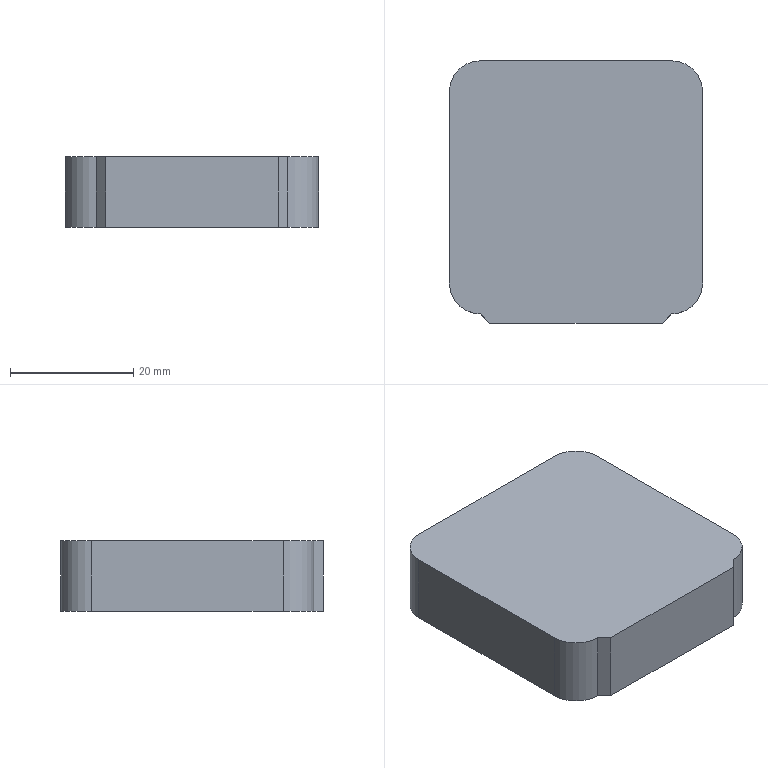Part | SolidWorks | features BaseBody 1 | 1 solid | 12 faces | box 41 x 42.5 x 11.5 mm | volume 19594 mm3 | plane 8 | cylinder 4 | commonest cylinder face diameters 10 x4
STEP:
#1=CARTESIAN_POINT('',(-10.199,-21.152,0.));
#2=VERTEX_POINT('',#1);
#3=CARTESIAN_POINT('',(17.801,-21.152,0.));
#4=VERTEX_POINT('',#3);
#5=CARTESIAN_POINT('',(3.801,-21.152,0.));
#6=DIRECTION('',(1.,0.,0.));
#7=VECTOR('',#6,1000.);
#8=LINE('',#5,#7);
#9=EDGE_CURVE('',#2,#4,#8,.T.);
#10=ORIENTED_EDGE('',*,*,#9,.F.);
#11=CARTESIAN_POINT('',(-11.699,-19.652,0.));
#12=VERTEX_POINT('',#11);
#13=CARTESIAN_POINT('',(-11.699,-19.652,0.));
#14=DIRECTION('',(0.7071,-0.7071,0.));
#15=VECTOR('',#14,1000.);
#16=LINE('',#13,#15);
#17=EDGE_CURVE('',#12,#2,#16,.T.);
#18=ORIENTED_EDGE('',*,*,#17,.F.);
#19=CARTESIAN_POINT('',(-16.699,-14.652,0.));
#20=VERTEX_POINT('',#19);
#21=CARTESIAN_POINT('',(-11.699,-14.652,0.));
#22=DIRECTION('',(0.,0.,1.));
#23=DIRECTION('',(1.,0.,0.));
#24=AXIS2_PLACEMENT_3D('',#21,#22,#23);
#25=CIRCLE('',#24,5.);
#26=EDGE_CURVE('',#20,#12,#25,.T.);
#27=ORIENTED_EDGE('',*,*,#26,.F.);
#28=CARTESIAN_POINT('',(-16.699,16.348,0.));
#29=VERTEX_POINT('',#28);
#30=CARTESIAN_POINT('',(-16.699,0.8485,0.));
#31=DIRECTION('',(0.,-1.,0.));
#32=VECTOR('',#31,1000.);
#33=LINE('',#30,#32);
#34=EDGE_CURVE('',#29,#20,#33,.T.);
#35=ORIENTED_EDGE('',*,*,#34,.F.);
#36=CARTESIAN_POINT('',(-11.699,21.348,0.));
#37=VERTEX_POINT('',#36);
#38=CARTESIAN_POINT('',(-11.699,16.348,0.));
#39=DIRECTION('',(0.,0.,1.));
#40=DIRECTION('',(1.,0.,0.));
#41=AXIS2_PLACEMENT_3D('',#38,#39,#40);
#42=CIRCLE('',#41,5.);
#43=EDGE_CURVE('',#37,#29,#42,.T.);
#44=ORIENTED_EDGE('',*,*,#43,.F.);
#45=CARTESIAN_POINT('',(19.301,21.348,0.));
#46=VERTEX_POINT('',#45);
#47=CARTESIAN_POINT('',(3.801,21.348,0.));
#48=DIRECTION('',(-1.,0.,0.));
#49=VECTOR('',#48,1000.);
#50=LINE('',#47,#49);
#51=EDGE_CURVE('',#46,#37,#50,.T.);
#52=ORIENTED_EDGE('',*,*,#51,.F.);
#53=CARTESIAN_POINT('',(24.301,16.348,0.));
#54=VERTEX_POINT('',#53);
#55=CARTESIAN_POINT('',(19.301,16.348,0.));
#56=DIRECTION('',(0.,0.,1.));
#57=DIRECTION('',(1.,0.,0.));
#58=AXIS2_PLACEMENT_3D('',#55,#56,#57);
#59=CIRCLE('',#58,5.);
#60=EDGE_CURVE('',#54,#46,#59,.T.);
#61=ORIENTED_EDGE('',*,*,#60,.F.);
#62=CARTESIAN_POINT('',(24.301,-14.652,0.));
#63=VERTEX_POINT('',#62);
#64=CARTESIAN_POINT('',(24.301,0.8485,0.));
#65=DIRECTION('',(0.,1.,0.));
#66=VECTOR('',#65,1000.);
#67=LINE('',#64,#66);
#68=EDGE_CURVE('',#63,#54,#67,.T.);
#69=ORIENTED_EDGE('',*,*,#68,.F.);
#70=CARTESIAN_POINT('',(19.301,-19.652,0.));
#71=VERTEX_POINT('',#70);
#72=CARTESIAN_POINT('',(19.301,-14.652,0.));
#73=DIRECTION('',(0.,0.,1.));
#74=DIRECTION('',(1.,0.,0.));
#75=AXIS2_PLACEMENT_3D('',#72,#73,#74);
#76=CIRCLE('',#75,5.);
#77=EDGE_CURVE('',#71,#63,#76,.T.);
#78=ORIENTED_EDGE('',*,*,#77,.F.);
#79=CARTESIAN_POINT('',(17.801,-21.152,0.));
#80=DIRECTION('',(0.7071,0.7071,0.));
#81=VECTOR('',#80,1000.);
#82=LINE('',#79,#81);
#83=EDGE_CURVE('',#4,#71,#82,.T.);
#84=ORIENTED_EDGE('',*,*,#83,.F.);
#85=EDGE_LOOP('',(#10,#18,#27,#35,#44,#52,#61,#69,#78,#84));
#86=FACE_OUTER_BOUND('',#85,.T.);
#87=CARTESIAN_POINT('',(3.801,0.8485,0.));
#88=DIRECTION('',(0.,0.,1.));
#89=DIRECTION('',(1.,0.,0.));
#90=AXIS2_PLACEMENT_3D('',#87,#88,#89);
#91=PLANE('',#90);
#92=ADVANCED_FACE('',(#86),#91,.F.);
#93=CARTESIAN_POINT('',(19.301,-19.652,11.5));
#94=VERTEX_POINT('',#93);
#95=CARTESIAN_POINT('',(17.801,-21.152,11.5));
#96=VERTEX_POINT('',#95);
#97=CARTESIAN_POINT('',(18.551,-20.402,11.5));
#98=DIRECTION('',(-0.7071,-0.7071,0.));
#99=VECTOR('',#98,1000.);
#100=LINE('',#97,#99);
#101=EDGE_CURVE('',#94,#96,#100,.T.);
#102=ORIENTED_EDGE('',*,*,#101,.T.);
#103=CARTESIAN_POINT('',(17.801,-21.152,8.625));
#104=DIRECTION('',(0.,0.,-1.));
#105=VECTOR('',#104,1000.);
#106=LINE('',#103,#105);
#107=EDGE_CURVE('',#96,#4,#106,.T.);
#108=ORIENTED_EDGE('',*,*,#107,.T.);
#109=ORIENTED_EDGE('',*,*,#83,.T.);
#110=CARTESIAN_POINT('',(19.301,-19.652,8.625));
#111=DIRECTION('',(0.,0.,1.));
#112=VECTOR('',#111,1000.);
#113=LINE('',#110,#112);
#114=EDGE_CURVE('',#71,#94,#113,.T.);
#115=ORIENTED_EDGE('',*,*,#114,.T.);
#116=EDGE_LOOP('',(#102,#108,#109,#115));
#117=FACE_OUTER_BOUND('',#116,.T.);
#118=CARTESIAN_POINT('',(18.551,-20.402,8.625));
#119=DIRECTION('',(0.7071,-0.7071,0.));
#120=DIRECTION('',(0.7071,0.7071,0.));
#121=AXIS2_PLACEMENT_3D('',#118,#119,#120);
#122=PLANE('',#121);
#123=ADVANCED_FACE('',(#117),#122,.T.);
#124=CARTESIAN_POINT('',(-10.199,-21.152,11.5));
#125=VERTEX_POINT('',#124);
#126=CARTESIAN_POINT('',(3.801,-21.152,11.5));
#127=DIRECTION('',(1.,0.,0.));
#128=VECTOR('',#127,1000.);
#129=LINE('',#126,#128);
#130=EDGE_CURVE('',#125,#96,#129,.T.);
#131=ORIENTED_EDGE('',*,*,#130,.F.);
#132=CARTESIAN_POINT('',(-10.199,-21.152,5.75));
#133=DIRECTION('',(0.,0.,1.));
#134=VECTOR('',#133,1000.);
#135=LINE('',#132,#134);
#136=EDGE_CURVE('',#2,#125,#135,.T.);
#137=ORIENTED_EDGE('',*,*,#136,.F.);
#138=ORIENTED_EDGE('',*,*,#9,.T.);
#139=ORIENTED_EDGE('',*,*,#107,.F.);
#140=EDGE_LOOP('',(#131,#137,#138,#139));
#141=FACE_OUTER_BOUND('',#140,.T.);
#142=CARTESIAN_POINT('',(3.801,-21.152,5.75));
#143=DIRECTION('',(0.,1.,0.));
#144=DIRECTION('',(0.,0.,1.));
#145=AXIS2_PLACEMENT_3D('',#142,#143,#144);
#146=PLANE('',#145);
#147=ADVANCED_FACE('',(#141),#146,.F.);
#148=ORIENTED_EDGE('',*,*,#17,.T.);
#149=ORIENTED_EDGE('',*,*,#136,.T.);
#150=CARTESIAN_POINT('',(-11.699,-19.652,11.5));
#151=VERTEX_POINT('',#150);
#152=CARTESIAN_POINT('',(-10.949,-20.402,11.5));
#153=DIRECTION('',(-0.7071,0.7071,0.));
#154=VECTOR('',#153,1000.);
#155=LINE('',#152,#154);
#156=EDGE_CURVE('',#125,#151,#155,.T.);
#157=ORIENTED_EDGE('',*,*,#156,.T.);
#158=CARTESIAN_POINT('',(-11.699,-19.652,2.875));
#159=DIRECTION('',(0.,0.,-1.));
#160=VECTOR('',#159,1000.);
#161=LINE('',#158,#160);
#162=EDGE_CURVE('',#151,#12,#161,.T.);
#163=ORIENTED_EDGE('',*,*,#162,.T.);
#164=EDGE_LOOP('',(#148,#149,#157,#163));
#165=FACE_OUTER_BOUND('',#164,.T.);
#166=CARTESIAN_POINT('',(-10.949,-20.402,2.875));
#167=DIRECTION('',(-0.7071,-0.7071,0.));
#168=DIRECTION('',(0.7071,-0.7071,0.));
#169=AXIS2_PLACEMENT_3D('',#166,#167,#168);
#170=PLANE('',#169);
#171=ADVANCED_FACE('',(#165),#170,.T.);
#172=ORIENTED_EDGE('',*,*,#26,.T.);
#173=ORIENTED_EDGE('',*,*,#162,.F.);
#174=CARTESIAN_POINT('',(-16.699,-14.652,11.5));
#175=VERTEX_POINT('',#174);
#176=CARTESIAN_POINT('',(-11.699,-14.652,11.5));
#177=DIRECTION('',(0.,0.,-1.));
#178=DIRECTION('',(1.,0.,0.));
#179=AXIS2_PLACEMENT_3D('',#176,#177,#178);
#180=CIRCLE('',#179,5.);
#181=EDGE_CURVE('',#151,#175,#180,.T.);
#182=ORIENTED_EDGE('',*,*,#181,.T.);
#183=CARTESIAN_POINT('',(-16.699,-14.652,0.));
#184=DIRECTION('',(0.,0.,-1.));
#185=VECTOR('',#184,1000.);
#186=LINE('',#183,#185);
#187=EDGE_CURVE('',#175,#20,#186,.T.);
#188=ORIENTED_EDGE('',*,*,#187,.T.);
#189=EDGE_LOOP('',(#172,#173,#182,#188));
#190=FACE_OUTER_BOUND('',#189,.T.);
#191=CARTESIAN_POINT('',(-11.699,-14.652,0.));
#192=DIRECTION('',(0.,0.,1.));
#193=DIRECTION('',(1.,0.,0.));
#194=AXIS2_PLACEMENT_3D('',#191,#192,#193);
#195=CYLINDRICAL_SURFACE('',#194,5.);
#196=ADVANCED_FACE('',(#190),#195,.T.);
#197=CARTESIAN_POINT('',(-16.699,16.348,11.5));
#198=VERTEX_POINT('',#197);
#199=CARTESIAN_POINT('',(-16.699,16.348,0.));
#200=DIRECTION('',(0.,0.,-1.));
#201=VECTOR('',#200,1000.);
#202=LINE('',#199,#201);
#203=EDGE_CURVE('',#198,#29,#202,.T.);
#204=ORIENTED_EDGE('',*,*,#203,.T.);
#205=ORIENTED_EDGE('',*,*,#34,.T.);
#206=ORIENTED_EDGE('',*,*,#187,.F.);
#207=CARTESIAN_POINT('',(-16.699,-19.652,11.5));
#208=DIRECTION('',(0.,1.,0.));
#209=VECTOR('',#208,1000.);
#210=LINE('',#207,#209);
#211=EDGE_CURVE('',#175,#198,#210,.T.);
#212=ORIENTED_EDGE('',*,*,#211,.T.);
#213=EDGE_LOOP('',(#204,#205,#206,#212));
#214=FACE_OUTER_BOUND('',#213,.T.);
#215=CARTESIAN_POINT('',(-16.699,-19.652,0.));
#216=DIRECTION('',(-1.,0.,0.));
#217=DIRECTION('',(0.,0.,1.));
#218=AXIS2_PLACEMENT_3D('',#215,#216,#217);
#219=PLANE('',#218);
#220=ADVANCED_FACE('',(#214),#219,.T.);
#221=ORIENTED_EDGE('',*,*,#43,.T.);
#222=ORIENTED_EDGE('',*,*,#203,.F.);
#223=CARTESIAN_POINT('',(-11.699,21.348,11.5));
#224=VERTEX_POINT('',#223);
#225=CARTESIAN_POINT('',(-11.699,16.348,11.5));
#226=DIRECTION('',(0.,0.,-1.));
#227=DIRECTION('',(1.,0.,0.));
#228=AXIS2_PLACEMENT_3D('',#225,#226,#227);
#229=CIRCLE('',#228,5.);
#230=EDGE_CURVE('',#198,#224,#229,.T.);
#231=ORIENTED_EDGE('',*,*,#230,.T.);
#232=CARTESIAN_POINT('',(-11.699,21.348,0.));
#233=DIRECTION('',(0.,0.,-1.));
#234=VECTOR('',#233,1000.);
#235=LINE('',#232,#234);
#236=EDGE_CURVE('',#224,#37,#235,.T.);
#237=ORIENTED_EDGE('',*,*,#236,.T.);
#238=EDGE_LOOP('',(#221,#222,#231,#237));
#239=FACE_OUTER_BOUND('',#238,.T.);
#240=CARTESIAN_POINT('',(-11.699,16.348,0.));
#241=DIRECTION('',(0.,0.,1.));
#242=DIRECTION('',(1.,0.,0.));
#243=AXIS2_PLACEMENT_3D('',#240,#241,#242);
#244=CYLINDRICAL_SURFACE('',#243,5.);
#245=ADVANCED_FACE('',(#239),#244,.T.);
#246=ORIENTED_EDGE('',*,*,#236,.F.);
#247=CARTESIAN_POINT('',(19.301,21.348,11.5));
#248=VERTEX_POINT('',#247);
#249=CARTESIAN_POINT('',(-16.699,21.348,11.5));
#250=DIRECTION('',(1.,0.,0.));
#251=VECTOR('',#250,1000.);
#252=LINE('',#249,#251);
#253=EDGE_CURVE('',#224,#248,#252,.T.);
#254=ORIENTED_EDGE('',*,*,#253,.T.);
#255=CARTESIAN_POINT('',(19.301,21.348,0.));
#256=DIRECTION('',(0.,0.,-1.));
#257=VECTOR('',#256,1000.);
#258=LINE('',#255,#257);
#259=EDGE_CURVE('',#248,#46,#258,.T.);
#260=ORIENTED_EDGE('',*,*,#259,.T.);
#261=ORIENTED_EDGE('',*,*,#51,.T.);
#262=EDGE_LOOP('',(#246,#254,#260,#261));
#263=FACE_OUTER_BOUND('',#262,.T.);
#264=CARTESIAN_POINT('',(-16.699,21.348,0.));
#265=DIRECTION('',(0.,1.,0.));
#266=DIRECTION('',(0.,0.,1.));
#267=AXIS2_PLACEMENT_3D('',#264,#265,#266);
#268=PLANE('',#267);
#269=ADVANCED_FACE('',(#263),#268,.T.);
#270=ORIENTED_EDGE('',*,*,#60,.T.);
#271=ORIENTED_EDGE('',*,*,#259,.F.);
#272=CARTESIAN_POINT('',(24.301,16.348,11.5));
#273=VERTEX_POINT('',#272);
#274=CARTESIAN_POINT('',(19.301,16.348,11.5));
#275=DIRECTION('',(0.,0.,-1.));
#276=DIRECTION('',(1.,0.,0.));
#277=AXIS2_PLACEMENT_3D('',#274,#275,#276);
#278=CIRCLE('',#277,5.);
#279=EDGE_CURVE('',#248,#273,#278,.T.);
#280=ORIENTED_EDGE('',*,*,#279,.T.);
#281=CARTESIAN_POINT('',(24.301,16.348,0.));
#282=DIRECTION('',(0.,0.,-1.));
#283=VECTOR('',#282,1000.);
#284=LINE('',#281,#283);
#285=EDGE_CURVE('',#273,#54,#284,.T.);
#286=ORIENTED_EDGE('',*,*,#285,.T.);
#287=EDGE_LOOP('',(#270,#271,#280,#286));
#288=FACE_OUTER_BOUND('',#287,.T.);
#289=CARTESIAN_POINT('',(19.301,16.348,0.));
#290=DIRECTION('',(0.,0.,1.));
#291=DIRECTION('',(1.,0.,0.));
#292=AXIS2_PLACEMENT_3D('',#289,#290,#291);
#293=CYLINDRICAL_SURFACE('',#292,5.);
#294=ADVANCED_FACE('',(#288),#293,.T.);
#295=ORIENTED_EDGE('',*,*,#285,.F.);
#296=CARTESIAN_POINT('',(24.301,-14.652,11.5));
#297=VERTEX_POINT('',#296);
#298=CARTESIAN_POINT('',(24.301,21.348,11.5));
#299=DIRECTION('',(0.,-1.,0.));
#300=VECTOR('',#299,1000.);
#301=LINE('',#298,#300);
#302=EDGE_CURVE('',#273,#297,#301,.T.);
#303=ORIENTED_EDGE('',*,*,#302,.T.);
#304=CARTESIAN_POINT('',(24.301,-14.652,0.));
#305=DIRECTION('',(0.,0.,-1.));
#306=VECTOR('',#305,1000.);
#307=LINE('',#304,#306);
#308=EDGE_CURVE('',#297,#63,#307,.T.);
#309=ORIENTED_EDGE('',*,*,#308,.T.);
#310=ORIENTED_EDGE('',*,*,#68,.T.);
#311=EDGE_LOOP('',(#295,#303,#309,#310));
#312=FACE_OUTER_BOUND('',#311,.T.);
#313=CARTESIAN_POINT('',(24.301,21.348,0.));
#314=DIRECTION('',(1.,0.,0.));
#315=DIRECTION('',(0.,0.,-1.));
#316=AXIS2_PLACEMENT_3D('',#313,#314,#315);
#317=PLANE('',#316);
#318=ADVANCED_FACE('',(#312),#317,.T.);
#319=ORIENTED_EDGE('',*,*,#77,.T.);
#320=ORIENTED_EDGE('',*,*,#308,.F.);
#321=CARTESIAN_POINT('',(19.301,-14.652,11.5));
#322=DIRECTION('',(0.,0.,-1.));
#323=DIRECTION('',(1.,0.,0.));
#324=AXIS2_PLACEMENT_3D('',#321,#322,#323);
#325=CIRCLE('',#324,5.);
#326=EDGE_CURVE('',#297,#94,#325,.T.);
#327=ORIENTED_EDGE('',*,*,#326,.T.);
#328=ORIENTED_EDGE('',*,*,#114,.F.);
#329=EDGE_LOOP('',(#319,#320,#327,#328));
#330=FACE_OUTER_BOUND('',#329,.T.);
#331=CARTESIAN_POINT('',(19.301,-14.652,0.));
#332=DIRECTION('',(0.,0.,1.));
#333=DIRECTION('',(1.,0.,0.));
#334=AXIS2_PLACEMENT_3D('',#331,#332,#333);
#335=CYLINDRICAL_SURFACE('',#334,5.);
#336=ADVANCED_FACE('',(#330),#335,.T.);
#337=ORIENTED_EDGE('',*,*,#156,.F.);
#338=ORIENTED_EDGE('',*,*,#130,.T.);
#339=ORIENTED_EDGE('',*,*,#101,.F.);
#340=ORIENTED_EDGE('',*,*,#326,.F.);
#341=ORIENTED_EDGE('',*,*,#302,.F.);
#342=ORIENTED_EDGE('',*,*,#279,.F.);
#343=ORIENTED_EDGE('',*,*,#253,.F.);
#344=ORIENTED_EDGE('',*,*,#230,.F.);
#345=ORIENTED_EDGE('',*,*,#211,.F.);
#346=ORIENTED_EDGE('',*,*,#181,.F.);
#347=EDGE_LOOP('',(#337,#338,#339,#340,#341,#342,#343,#344,#345,#346));
#348=FACE_OUTER_BOUND('',#347,.T.);
#349=CARTESIAN_POINT('',(3.801,0.8485,11.5));
#350=DIRECTION('',(0.,0.,1.));
#351=DIRECTION('',(1.,0.,0.));
#352=AXIS2_PLACEMENT_3D('',#349,#350,#351);
#353=PLANE('',#352);
#354=ADVANCED_FACE('',(#348),#353,.T.);
#355=CLOSED_SHELL('',(#92,#123,#147,#171,#196,#220,#245,#269,#294,#318,#336,#354));
#356=MANIFOLD_SOLID_BREP('',#355);
#357=CARTESIAN_POINT('',(0.,0.,0.));
#358=DIRECTION('',(0.,0.,1.));
#359=DIRECTION('',(1.,0.,0.));
#360=AXIS2_PLACEMENT_3D('',#357,#358,#359);
#361=(LENGTH_UNIT()NAMED_UNIT(*)SI_UNIT(.MILLI.,.METRE.));
#362=UNCERTAINTY_MEASURE_WITH_UNIT(LENGTH_MEASURE(0.00001),#361,'','');
#363=(NAMED_UNIT(*)PLANE_ANGLE_UNIT()SI_UNIT($,.RADIAN.));
#364=(NAMED_UNIT(*)SI_UNIT($,.STERADIAN.)SOLID_ANGLE_UNIT());
#365=(GEOMETRIC_REPRESENTATION_CONTEXT(3)GLOBAL_UNCERTAINTY_ASSIGNED_CONTEXT((#362))GLOBAL_UNIT_ASSIGNED_CONTEXT((#361,#363,#364))REPRESENTATION_CONTEXT('',''));
#366=ADVANCED_BREP_SHAPE_REPRESENTATION('',(#356,#360),#365);